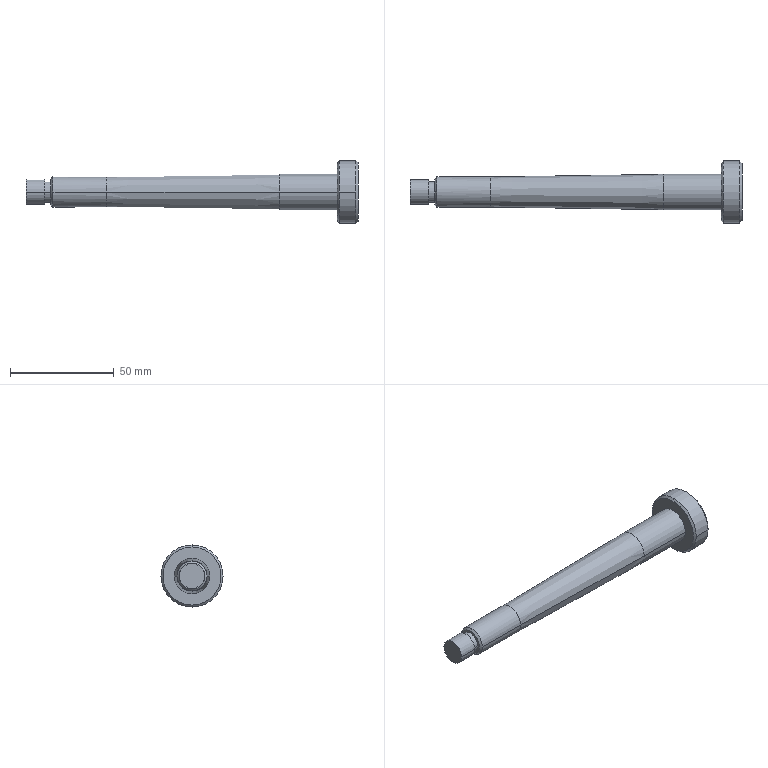Part | SolidWorks | features Chamfer 1, Revolution 1 | 1 solid | 23 faces | box 160 x 30 x 30 mm | volume 35227 mm3 | cylinder 10 | cone 8 | plane 5 | commonest cylinder face diameters 10 x2 12 x2 14.5 x2 17 x2 30 x2
STEP:
#1=CARTESIAN_POINT('',(272.45,-57.118,14.));
#2=VERTEX_POINT('',#1);
#3=CARTESIAN_POINT('',(272.45,-57.118,-14.));
#4=VERTEX_POINT('',#3);
#5=CARTESIAN_POINT('',(272.45,-57.118,0.));
#6=DIRECTION('',(-1.,0.,0.));
#7=DIRECTION('',(0.,-1.,0.));
#8=AXIS2_PLACEMENT_3D('',#5,#6,#7);
#9=CIRCLE('',#8,14.);
#10=EDGE_CURVE('',#2,#4,#9,.T.);
#11=ORIENTED_EDGE('',*,*,#10,.F.);
#12=CARTESIAN_POINT('',(273.45,-57.118,15.));
#13=VERTEX_POINT('',#12);
#14=CARTESIAN_POINT('',(273.45,-57.118,15.));
#15=DIRECTION('',(0.7071,0.,0.7071));
#16=VECTOR('',#15,1000.);
#17=LINE('',#14,#16);
#18=EDGE_CURVE('',#2,#13,#17,.T.);
#19=ORIENTED_EDGE('',*,*,#18,.T.);
#20=CARTESIAN_POINT('',(273.45,-42.118,0.));
#21=VERTEX_POINT('',#20);
#22=CARTESIAN_POINT('',(273.45,-57.118,0.));
#23=DIRECTION('',(1.,0.,0.));
#24=DIRECTION('',(0.,0.,1.));
#25=AXIS2_PLACEMENT_3D('',#22,#23,#24);
#26=CIRCLE('',#25,15.);
#27=EDGE_CURVE('',#21,#13,#26,.T.);
#28=ORIENTED_EDGE('',*,*,#27,.F.);
#29=CARTESIAN_POINT('',(273.45,-57.118,-15.));
#30=VERTEX_POINT('',#29);
#31=CARTESIAN_POINT('',(273.45,-57.118,0.));
#32=DIRECTION('',(1.,0.,0.));
#33=DIRECTION('',(0.,0.,1.));
#34=AXIS2_PLACEMENT_3D('',#31,#32,#33);
#35=CIRCLE('',#34,15.);
#36=EDGE_CURVE('',#30,#21,#35,.T.);
#37=ORIENTED_EDGE('',*,*,#36,.F.);
#38=CARTESIAN_POINT('',(273.45,-57.118,-15.));
#39=DIRECTION('',(0.7071,0.,-0.7071));
#40=VECTOR('',#39,1000.);
#41=LINE('',#38,#40);
#42=EDGE_CURVE('',#4,#30,#41,.T.);
#43=ORIENTED_EDGE('',*,*,#42,.F.);
#44=EDGE_LOOP('',(#11,#19,#28,#37,#43));
#45=FACE_OUTER_BOUND('',#44,.T.);
#46=CARTESIAN_POINT('',(273.45,-57.118,0.));
#47=DIRECTION('',(1.,0.,0.));
#48=DIRECTION('',(0.,0.,-1.));
#49=AXIS2_PLACEMENT_3D('',#46,#47,#48);
#50=CONICAL_SURFACE('',#49,15.,0.7854);
#51=ADVANCED_FACE('',(#45),#50,.T.);
#52=CARTESIAN_POINT('',(282.45,-57.118,-14.));
#53=VERTEX_POINT('',#52);
#54=CARTESIAN_POINT('',(282.45,-57.118,14.));
#55=VERTEX_POINT('',#54);
#56=CARTESIAN_POINT('',(282.45,-57.118,0.));
#57=DIRECTION('',(1.,0.,0.));
#58=DIRECTION('',(0.,1.,0.));
#59=AXIS2_PLACEMENT_3D('',#56,#57,#58);
#60=CIRCLE('',#59,14.);
#61=EDGE_CURVE('',#53,#55,#60,.T.);
#62=ORIENTED_EDGE('',*,*,#61,.F.);
#63=CARTESIAN_POINT('',(281.45,-57.118,-15.));
#64=VERTEX_POINT('',#63);
#65=CARTESIAN_POINT('',(282.45,-57.118,-14.));
#66=DIRECTION('',(-0.7071,0.,-0.7071));
#67=VECTOR('',#66,1000.);
#68=LINE('',#65,#67);
#69=EDGE_CURVE('',#53,#64,#68,.T.);
#70=ORIENTED_EDGE('',*,*,#69,.T.);
#71=CARTESIAN_POINT('',(281.45,-42.118,0.));
#72=VERTEX_POINT('',#71);
#73=CARTESIAN_POINT('',(281.45,-57.118,0.));
#74=DIRECTION('',(-1.,0.,0.));
#75=DIRECTION('',(0.,0.,-1.));
#76=AXIS2_PLACEMENT_3D('',#73,#74,#75);
#77=CIRCLE('',#76,15.);
#78=EDGE_CURVE('',#72,#64,#77,.T.);
#79=ORIENTED_EDGE('',*,*,#78,.F.);
#80=CARTESIAN_POINT('',(281.45,-57.118,15.));
#81=VERTEX_POINT('',#80);
#82=CARTESIAN_POINT('',(281.45,-57.118,0.));
#83=DIRECTION('',(-1.,0.,0.));
#84=DIRECTION('',(0.,0.,-1.));
#85=AXIS2_PLACEMENT_3D('',#82,#83,#84);
#86=CIRCLE('',#85,15.);
#87=EDGE_CURVE('',#81,#72,#86,.T.);
#88=ORIENTED_EDGE('',*,*,#87,.F.);
#89=CARTESIAN_POINT('',(282.45,-57.118,14.));
#90=DIRECTION('',(-0.7071,0.,0.7071));
#91=VECTOR('',#90,1000.);
#92=LINE('',#89,#91);
#93=EDGE_CURVE('',#55,#81,#92,.T.);
#94=ORIENTED_EDGE('',*,*,#93,.F.);
#95=EDGE_LOOP('',(#62,#70,#79,#88,#94));
#96=FACE_OUTER_BOUND('',#95,.T.);
#97=CARTESIAN_POINT('',(282.45,-57.118,0.));
#98=DIRECTION('',(-1.,0.,0.));
#99=DIRECTION('',(0.,0.,1.));
#100=AXIS2_PLACEMENT_3D('',#97,#98,#99);
#101=CONICAL_SURFACE('',#100,14.,0.7854);
#102=ADVANCED_FACE('',(#96),#101,.T.);
#103=CARTESIAN_POINT('',(134.45,-57.118,6.25));
#104=VERTEX_POINT('',#103);
#105=CARTESIAN_POINT('',(134.45,-57.118,-6.25));
#106=VERTEX_POINT('',#105);
#107=CARTESIAN_POINT('',(134.45,-57.118,0.));
#108=DIRECTION('',(-1.,0.,0.));
#109=DIRECTION('',(0.,-1.,0.));
#110=AXIS2_PLACEMENT_3D('',#107,#108,#109);
#111=CIRCLE('',#110,6.25);
#112=EDGE_CURVE('',#104,#106,#111,.T.);
#113=ORIENTED_EDGE('',*,*,#112,.F.);
#114=CARTESIAN_POINT('',(135.45,-57.118,7.25));
#115=VERTEX_POINT('',#114);
#116=CARTESIAN_POINT('',(135.45,-57.118,7.25));
#117=DIRECTION('',(0.7071,0.,0.7071));
#118=VECTOR('',#117,1000.);
#119=LINE('',#116,#118);
#120=EDGE_CURVE('',#104,#115,#119,.T.);
#121=ORIENTED_EDGE('',*,*,#120,.T.);
#122=CARTESIAN_POINT('',(135.45,-49.868,0.));
#123=VERTEX_POINT('',#122);
#124=CARTESIAN_POINT('',(135.45,-57.118,0.));
#125=DIRECTION('',(1.,0.,0.));
#126=DIRECTION('',(0.,0.,1.));
#127=AXIS2_PLACEMENT_3D('',#124,#125,#126);
#128=CIRCLE('',#127,7.25);
#129=EDGE_CURVE('',#123,#115,#128,.T.);
#130=ORIENTED_EDGE('',*,*,#129,.F.);
#131=CARTESIAN_POINT('',(135.45,-57.118,-7.25));
#132=VERTEX_POINT('',#131);
#133=CARTESIAN_POINT('',(135.45,-57.118,0.));
#134=DIRECTION('',(1.,0.,0.));
#135=DIRECTION('',(0.,0.,1.));
#136=AXIS2_PLACEMENT_3D('',#133,#134,#135);
#137=CIRCLE('',#136,7.25);
#138=EDGE_CURVE('',#132,#123,#137,.T.);
#139=ORIENTED_EDGE('',*,*,#138,.F.);
#140=CARTESIAN_POINT('',(135.45,-57.118,-7.25));
#141=DIRECTION('',(0.7071,0.,-0.7071));
#142=VECTOR('',#141,1000.);
#143=LINE('',#140,#142);
#144=EDGE_CURVE('',#106,#132,#143,.T.);
#145=ORIENTED_EDGE('',*,*,#144,.F.);
#146=EDGE_LOOP('',(#113,#121,#130,#139,#145));
#147=FACE_OUTER_BOUND('',#146,.T.);
#148=CARTESIAN_POINT('',(135.45,-57.118,0.));
#149=DIRECTION('',(1.,0.,0.));
#150=DIRECTION('',(0.,0.,-1.));
#151=AXIS2_PLACEMENT_3D('',#148,#149,#150);
#152=CONICAL_SURFACE('',#151,7.25,0.7854);
#153=ADVANCED_FACE('',(#147),#152,.T.);
#154=CARTESIAN_POINT('',(131.45,-52.118,0.));
#155=VERTEX_POINT('',#154);
#156=CARTESIAN_POINT('',(131.45,-62.118,0.));
#157=VERTEX_POINT('',#156);
#158=CARTESIAN_POINT('',(131.45,-57.118,0.));
#159=DIRECTION('',(1.,0.,0.));
#160=DIRECTION('',(0.,1.,0.));
#161=AXIS2_PLACEMENT_3D('',#158,#159,#160);
#162=CIRCLE('',#161,5.);
#163=EDGE_CURVE('',#155,#157,#162,.T.);
#164=ORIENTED_EDGE('',*,*,#163,.T.);
#165=CARTESIAN_POINT('',(134.45,-62.118,0.));
#166=VERTEX_POINT('',#165);
#167=CARTESIAN_POINT('',(272.45,-62.118,0.));
#168=DIRECTION('',(1.,0.,0.));
#169=VECTOR('',#168,1000.);
#170=LINE('',#167,#169);
#171=EDGE_CURVE('',#157,#166,#170,.T.);
#172=ORIENTED_EDGE('',*,*,#171,.T.);
#173=CARTESIAN_POINT('',(134.45,-52.118,0.));
#174=VERTEX_POINT('',#173);
#175=CARTESIAN_POINT('',(134.45,-57.118,0.));
#176=DIRECTION('',(1.,0.,0.));
#177=DIRECTION('',(0.,1.,0.));
#178=AXIS2_PLACEMENT_3D('',#175,#176,#177);
#179=CIRCLE('',#178,5.);
#180=EDGE_CURVE('',#174,#166,#179,.T.);
#181=ORIENTED_EDGE('',*,*,#180,.F.);
#182=CARTESIAN_POINT('',(272.45,-52.118,0.));
#183=DIRECTION('',(1.,0.,0.));
#184=VECTOR('',#183,1000.);
#185=LINE('',#182,#184);
#186=EDGE_CURVE('',#155,#174,#185,.T.);
#187=ORIENTED_EDGE('',*,*,#186,.F.);
#188=EDGE_LOOP('',(#164,#172,#181,#187));
#189=FACE_OUTER_BOUND('',#188,.T.);
#190=CARTESIAN_POINT('',(272.45,-57.118,0.));
#191=DIRECTION('',(1.,0.,0.));
#192=DIRECTION('',(0.,1.,0.));
#193=AXIS2_PLACEMENT_3D('',#190,#191,#192);
#194=CYLINDRICAL_SURFACE('',#193,5.);
#195=ADVANCED_FACE('',(#189),#194,.T.);
#196=CARTESIAN_POINT('',(122.45,-51.118,0.));
#197=VERTEX_POINT('',#196);
#198=CARTESIAN_POINT('',(122.45,-63.118,0.));
#199=VERTEX_POINT('',#198);
#200=CARTESIAN_POINT('',(122.45,-57.118,0.));
#201=DIRECTION('',(1.,0.,0.));
#202=DIRECTION('',(0.,1.,0.));
#203=AXIS2_PLACEMENT_3D('',#200,#201,#202);
#204=CIRCLE('',#203,6.);
#205=EDGE_CURVE('',#197,#199,#204,.T.);
#206=ORIENTED_EDGE('',*,*,#205,.T.);
#207=CARTESIAN_POINT('',(131.45,-63.118,0.));
#208=VERTEX_POINT('',#207);
#209=CARTESIAN_POINT('',(272.45,-63.118,0.));
#210=DIRECTION('',(1.,0.,0.));
#211=VECTOR('',#210,1000.);
#212=LINE('',#209,#211);
#213=EDGE_CURVE('',#199,#208,#212,.T.);
#214=ORIENTED_EDGE('',*,*,#213,.T.);
#215=CARTESIAN_POINT('',(131.45,-51.118,0.));
#216=VERTEX_POINT('',#215);
#217=CARTESIAN_POINT('',(131.45,-57.118,0.));
#218=DIRECTION('',(1.,0.,0.));
#219=DIRECTION('',(0.,1.,0.));
#220=AXIS2_PLACEMENT_3D('',#217,#218,#219);
#221=CIRCLE('',#220,6.);
#222=EDGE_CURVE('',#216,#208,#221,.T.);
#223=ORIENTED_EDGE('',*,*,#222,.F.);
#224=CARTESIAN_POINT('',(272.45,-51.118,0.));
#225=DIRECTION('',(1.,0.,0.));
#226=VECTOR('',#225,1000.);
#227=LINE('',#224,#226);
#228=EDGE_CURVE('',#197,#216,#227,.T.);
#229=ORIENTED_EDGE('',*,*,#228,.F.);
#230=EDGE_LOOP('',(#206,#214,#223,#229));
#231=FACE_OUTER_BOUND('',#230,.T.);
#232=CARTESIAN_POINT('',(272.45,-57.118,0.));
#233=DIRECTION('',(1.,0.,0.));
#234=DIRECTION('',(0.,1.,0.));
#235=AXIS2_PLACEMENT_3D('',#232,#233,#234);
#236=CYLINDRICAL_SURFACE('',#235,6.);
#237=ADVANCED_FACE('',(#231),#236,.T.);
#238=ORIENTED_EDGE('',*,*,#27,.T.);
#239=CARTESIAN_POINT('',(273.45,-72.118,0.));
#240=VERTEX_POINT('',#239);
#241=CARTESIAN_POINT('',(273.45,-57.118,0.));
#242=DIRECTION('',(1.,0.,0.));
#243=DIRECTION('',(0.,0.,1.));
#244=AXIS2_PLACEMENT_3D('',#241,#242,#243);
#245=CIRCLE('',#244,15.);
#246=EDGE_CURVE('',#13,#240,#245,.T.);
#247=ORIENTED_EDGE('',*,*,#246,.T.);
#248=CARTESIAN_POINT('',(281.45,-72.118,0.));
#249=VERTEX_POINT('',#248);
#250=CARTESIAN_POINT('',(272.45,-72.118,0.));
#251=DIRECTION('',(1.,0.,0.));
#252=VECTOR('',#251,1000.);
#253=LINE('',#250,#252);
#254=EDGE_CURVE('',#240,#249,#253,.T.);
#255=ORIENTED_EDGE('',*,*,#254,.T.);
#256=CARTESIAN_POINT('',(281.45,-57.118,0.));
#257=DIRECTION('',(-1.,0.,0.));
#258=DIRECTION('',(0.,0.,-1.));
#259=AXIS2_PLACEMENT_3D('',#256,#257,#258);
#260=CIRCLE('',#259,15.);
#261=EDGE_CURVE('',#249,#81,#260,.T.);
#262=ORIENTED_EDGE('',*,*,#261,.T.);
#263=ORIENTED_EDGE('',*,*,#87,.T.);
#264=CARTESIAN_POINT('',(272.45,-42.118,0.));
#265=DIRECTION('',(1.,0.,0.));
#266=VECTOR('',#265,1000.);
#267=LINE('',#264,#266);
#268=EDGE_CURVE('',#21,#72,#267,.T.);
#269=ORIENTED_EDGE('',*,*,#268,.F.);
#270=EDGE_LOOP('',(#238,#247,#255,#262,#263,#269));
#271=FACE_OUTER_BOUND('',#270,.T.);
#272=CARTESIAN_POINT('',(272.45,-57.118,0.));
#273=DIRECTION('',(1.,0.,0.));
#274=DIRECTION('',(0.,1.,0.));
#275=AXIS2_PLACEMENT_3D('',#272,#273,#274);
#276=CYLINDRICAL_SURFACE('',#275,15.);
#277=ADVANCED_FACE('',(#271),#276,.T.);
#278=CARTESIAN_POINT('',(244.45,-48.618,0.));
#279=VERTEX_POINT('',#278);
#280=CARTESIAN_POINT('',(244.45,-65.618,0.));
#281=VERTEX_POINT('',#280);
#282=CARTESIAN_POINT('',(244.45,-57.118,0.));
#283=DIRECTION('',(1.,0.,0.));
#284=DIRECTION('',(0.,1.,0.));
#285=AXIS2_PLACEMENT_3D('',#282,#283,#284);
#286=CIRCLE('',#285,8.5);
#287=EDGE_CURVE('',#279,#281,#286,.T.);
#288=ORIENTED_EDGE('',*,*,#287,.T.);
#289=CARTESIAN_POINT('',(272.45,-65.618,0.));
#290=VERTEX_POINT('',#289);
#291=CARTESIAN_POINT('',(272.45,-65.618,0.));
#292=DIRECTION('',(1.,0.,0.));
#293=VECTOR('',#292,1000.);
#294=LINE('',#291,#293);
#295=EDGE_CURVE('',#281,#290,#294,.T.);
#296=ORIENTED_EDGE('',*,*,#295,.T.);
#297=CARTESIAN_POINT('',(272.45,-48.618,0.));
#298=VERTEX_POINT('',#297);
#299=CARTESIAN_POINT('',(272.45,-57.118,0.));
#300=DIRECTION('',(1.,0.,0.));
#301=DIRECTION('',(0.,1.,0.));
#302=AXIS2_PLACEMENT_3D('',#299,#300,#301);
#303=CIRCLE('',#302,8.5);
#304=EDGE_CURVE('',#298,#290,#303,.T.);
#305=ORIENTED_EDGE('',*,*,#304,.F.);
#306=CARTESIAN_POINT('',(272.45,-48.618,0.));
#307=DIRECTION('',(1.,0.,0.));
#308=VECTOR('',#307,1000.);
#309=LINE('',#306,#308);
#310=EDGE_CURVE('',#279,#298,#309,.T.);
#311=ORIENTED_EDGE('',*,*,#310,.F.);
#312=EDGE_LOOP('',(#288,#296,#305,#311));
#313=FACE_OUTER_BOUND('',#312,.T.);
#314=CARTESIAN_POINT('',(272.45,-57.118,0.));
#315=DIRECTION('',(1.,0.,0.));
#316=DIRECTION('',(0.,1.,0.));
#317=AXIS2_PLACEMENT_3D('',#314,#315,#316);
#318=CYLINDRICAL_SURFACE('',#317,8.5);
#319=ADVANCED_FACE('',(#313),#318,.T.);
#320=CARTESIAN_POINT('',(161.45,-49.868,0.));
#321=VERTEX_POINT('',#320);
#322=CARTESIAN_POINT('',(161.45,-64.368,0.));
#323=VERTEX_POINT('',#322);
#324=CARTESIAN_POINT('',(161.45,-57.118,0.));
#325=DIRECTION('',(1.,0.,0.));
#326=DIRECTION('',(0.,1.,0.));
#327=AXIS2_PLACEMENT_3D('',#324,#325,#326);
#328=CIRCLE('',#327,7.25);
#329=EDGE_CURVE('',#321,#323,#328,.T.);
#330=ORIENTED_EDGE('',*,*,#329,.T.);
#331=CARTESIAN_POINT('',(244.45,-65.618,0.));
#332=DIRECTION('',(0.9999,-0.01506,0.));
#333=VECTOR('',#332,1000.);
#334=LINE('',#331,#333);
#335=EDGE_CURVE('',#323,#281,#334,.T.);
#336=ORIENTED_EDGE('',*,*,#335,.T.);
#337=ORIENTED_EDGE('',*,*,#287,.F.);
#338=CARTESIAN_POINT('',(244.45,-48.618,0.));
#339=DIRECTION('',(0.9999,0.01506,0.));
#340=VECTOR('',#339,1000.);
#341=LINE('',#338,#340);
#342=EDGE_CURVE('',#321,#279,#341,.T.);
#343=ORIENTED_EDGE('',*,*,#342,.F.);
#344=EDGE_LOOP('',(#330,#336,#337,#343));
#345=FACE_OUTER_BOUND('',#344,.T.);
#346=CARTESIAN_POINT('',(244.45,-57.118,0.));
#347=DIRECTION('',(1.,0.,0.));
#348=DIRECTION('',(0.,1.,0.));
#349=AXIS2_PLACEMENT_3D('',#346,#347,#348);
#350=CONICAL_SURFACE('',#349,8.5,0.01506);
#351=ADVANCED_FACE('',(#345),#350,.T.);
#352=ORIENTED_EDGE('',*,*,#129,.T.);
#353=CARTESIAN_POINT('',(135.45,-64.368,0.));
#354=VERTEX_POINT('',#353);
#355=CARTESIAN_POINT('',(135.45,-57.118,0.));
#356=DIRECTION('',(1.,0.,0.));
#357=DIRECTION('',(0.,0.,1.));
#358=AXIS2_PLACEMENT_3D('',#355,#356,#357);
#359=CIRCLE('',#358,7.25);
#360=EDGE_CURVE('',#115,#354,#359,.T.);
#361=ORIENTED_EDGE('',*,*,#360,.T.);
#362=CARTESIAN_POINT('',(272.45,-64.368,0.));
#363=DIRECTION('',(1.,0.,0.));
#364=VECTOR('',#363,1000.);
#365=LINE('',#362,#364);
#366=EDGE_CURVE('',#354,#323,#365,.T.);
#367=ORIENTED_EDGE('',*,*,#366,.T.);
#368=ORIENTED_EDGE('',*,*,#329,.F.);
#369=CARTESIAN_POINT('',(272.45,-49.868,0.));
#370=DIRECTION('',(1.,0.,0.));
#371=VECTOR('',#370,1000.);
#372=LINE('',#369,#371);
#373=EDGE_CURVE('',#123,#321,#372,.T.);
#374=ORIENTED_EDGE('',*,*,#373,.F.);
#375=EDGE_LOOP('',(#352,#361,#367,#368,#374));
#376=FACE_OUTER_BOUND('',#375,.T.);
#377=CARTESIAN_POINT('',(272.45,-57.118,0.));
#378=DIRECTION('',(1.,0.,0.));
#379=DIRECTION('',(0.,1.,0.));
#380=AXIS2_PLACEMENT_3D('',#377,#378,#379);
#381=CYLINDRICAL_SURFACE('',#380,7.25);
#382=ADVANCED_FACE('',(#376),#381,.T.);
#383=CARTESIAN_POINT('',(134.45,-57.118,0.));
#384=DIRECTION('',(-1.,0.,0.));
#385=DIRECTION('',(0.,-1.,0.));
#386=AXIS2_PLACEMENT_3D('',#383,#384,#385);
#387=CIRCLE('',#386,6.25);
#388=EDGE_CURVE('',#106,#104,#387,.T.);
#389=ORIENTED_EDGE('',*,*,#388,.T.);
#390=ORIENTED_EDGE('',*,*,#112,.T.);
#391=EDGE_LOOP('',(#389,#390));
#392=FACE_OUTER_BOUND('',#391,.T.);
#393=ORIENTED_EDGE('',*,*,#180,.T.);
#394=CARTESIAN_POINT('',(134.45,-57.118,0.));
#395=DIRECTION('',(1.,0.,0.));
#396=DIRECTION('',(0.,1.,0.));
#397=AXIS2_PLACEMENT_3D('',#394,#395,#396);
#398=CIRCLE('',#397,5.);
#399=EDGE_CURVE('',#166,#174,#398,.T.);
#400=ORIENTED_EDGE('',*,*,#399,.T.);
#401=EDGE_LOOP('',(#393,#400));
#402=FACE_BOUND('',#401,.T.);
#403=CARTESIAN_POINT('',(134.45,-49.868,0.));
#404=DIRECTION('',(-1.,0.,0.));
#405=DIRECTION('',(0.,-1.,0.));
#406=AXIS2_PLACEMENT_3D('',#403,#404,#405);
#407=PLANE('',#406);
#408=ADVANCED_FACE('',(#392,#402),#407,.T.);
#409=ORIENTED_EDGE('',*,*,#366,.F.);
#410=CARTESIAN_POINT('',(135.45,-57.118,0.));
#411=DIRECTION('',(1.,0.,0.));
#412=DIRECTION('',(0.,0.,1.));
#413=AXIS2_PLACEMENT_3D('',#410,#411,#412);
#414=CIRCLE('',#413,7.25);
#415=EDGE_CURVE('',#354,#132,#414,.T.);
#416=ORIENTED_EDGE('',*,*,#415,.T.);
#417=ORIENTED_EDGE('',*,*,#138,.T.);
#418=ORIENTED_EDGE('',*,*,#373,.T.);
#419=CARTESIAN_POINT('',(161.45,-57.118,0.));
#420=DIRECTION('',(1.,0.,0.));
#421=DIRECTION('',(0.,1.,0.));
#422=AXIS2_PLACEMENT_3D('',#419,#420,#421);
#423=CIRCLE('',#422,7.25);
#424=EDGE_CURVE('',#323,#321,#423,.T.);
#425=ORIENTED_EDGE('',*,*,#424,.F.);
#426=EDGE_LOOP('',(#409,#416,#417,#418,#425));
#427=FACE_OUTER_BOUND('',#426,.T.);
#428=CARTESIAN_POINT('',(272.45,-57.118,0.));
#429=DIRECTION('',(1.,0.,0.));
#430=DIRECTION('',(0.,1.,0.));
#431=AXIS2_PLACEMENT_3D('',#428,#429,#430);
#432=CYLINDRICAL_SURFACE('',#431,7.25);
#433=ADVANCED_FACE('',(#427),#432,.T.);
#434=ORIENTED_EDGE('',*,*,#335,.F.);
#435=ORIENTED_EDGE('',*,*,#424,.T.);
#436=ORIENTED_EDGE('',*,*,#342,.T.);
#437=CARTESIAN_POINT('',(244.45,-57.118,0.));
#438=DIRECTION('',(1.,0.,0.));
#439=DIRECTION('',(0.,1.,0.));
#440=AXIS2_PLACEMENT_3D('',#437,#438,#439);
#441=CIRCLE('',#440,8.5);
#442=EDGE_CURVE('',#281,#279,#441,.T.);
#443=ORIENTED_EDGE('',*,*,#442,.F.);
#444=EDGE_LOOP('',(#434,#435,#436,#443));
#445=FACE_OUTER_BOUND('',#444,.T.);
#446=CARTESIAN_POINT('',(244.45,-57.118,0.));
#447=DIRECTION('',(1.,0.,0.));
#448=DIRECTION('',(0.,1.,0.));
#449=AXIS2_PLACEMENT_3D('',#446,#447,#448);
#450=CONICAL_SURFACE('',#449,8.5,0.01506);
#451=ADVANCED_FACE('',(#445),#450,.T.);
#452=ORIENTED_EDGE('',*,*,#295,.F.);
#453=ORIENTED_EDGE('',*,*,#442,.T.);
#454=ORIENTED_EDGE('',*,*,#310,.T.);
#455=CARTESIAN_POINT('',(272.45,-57.118,0.));
#456=DIRECTION('',(1.,0.,0.));
#457=DIRECTION('',(0.,1.,0.));
#458=AXIS2_PLACEMENT_3D('',#455,#456,#457);
#459=CIRCLE('',#458,8.5);
#460=EDGE_CURVE('',#290,#298,#459,.T.);
#461=ORIENTED_EDGE('',*,*,#460,.F.);
#462=EDGE_LOOP('',(#452,#453,#454,#461));
#463=FACE_OUTER_BOUND('',#462,.T.);
#464=CARTESIAN_POINT('',(272.45,-57.118,0.));
#465=DIRECTION('',(1.,0.,0.));
#466=DIRECTION('',(0.,1.,0.));
#467=AXIS2_PLACEMENT_3D('',#464,#465,#466);
#468=CYLINDRICAL_SURFACE('',#467,8.5);
#469=ADVANCED_FACE('',(#463),#468,.T.);
#470=CARTESIAN_POINT('',(272.45,-57.118,0.));
#471=DIRECTION('',(-1.,0.,0.));
#472=DIRECTION('',(0.,-1.,0.));
#473=AXIS2_PLACEMENT_3D('',#470,#471,#472);
#474=CIRCLE('',#473,14.);
#475=EDGE_CURVE('',#4,#2,#474,.T.);
#476=ORIENTED_EDGE('',*,*,#475,.T.);
#477=ORIENTED_EDGE('',*,*,#10,.T.);
#478=EDGE_LOOP('',(#476,#477));
#479=FACE_OUTER_BOUND('',#478,.T.);
#480=ORIENTED_EDGE('',*,*,#304,.T.);
#481=ORIENTED_EDGE('',*,*,#460,.T.);
#482=EDGE_LOOP('',(#480,#481));
#483=FACE_BOUND('',#482,.T.);
#484=CARTESIAN_POINT('',(272.45,-48.618,0.));
#485=DIRECTION('',(-1.,0.,0.));
#486=DIRECTION('',(0.,-1.,0.));
#487=AXIS2_PLACEMENT_3D('',#484,#485,#486);
#488=PLANE('',#487);
#489=ADVANCED_FACE('',(#479,#483),#488,.T.);
#490=ORIENTED_EDGE('',*,*,#254,.F.);
#491=CARTESIAN_POINT('',(273.45,-57.118,0.));
#492=DIRECTION('',(1.,0.,0.));
#493=DIRECTION('',(0.,0.,1.));
#494=AXIS2_PLACEMENT_3D('',#491,#492,#493);
#495=CIRCLE('',#494,15.);
#496=EDGE_CURVE('',#240,#30,#495,.T.);
#497=ORIENTED_EDGE('',*,*,#496,.T.);
#498=ORIENTED_EDGE('',*,*,#36,.T.);
#499=ORIENTED_EDGE('',*,*,#268,.T.);
#500=ORIENTED_EDGE('',*,*,#78,.T.);
#501=CARTESIAN_POINT('',(281.45,-57.118,0.));
#502=DIRECTION('',(-1.,0.,0.));
#503=DIRECTION('',(0.,0.,-1.));
#504=AXIS2_PLACEMENT_3D('',#501,#502,#503);
#505=CIRCLE('',#504,15.);
#506=EDGE_CURVE('',#64,#249,#505,.T.);
#507=ORIENTED_EDGE('',*,*,#506,.T.);
#508=EDGE_LOOP('',(#490,#497,#498,#499,#500,#507));
#509=FACE_OUTER_BOUND('',#508,.T.);
#510=CARTESIAN_POINT('',(272.45,-57.118,0.));
#511=DIRECTION('',(1.,0.,0.));
#512=DIRECTION('',(0.,1.,0.));
#513=AXIS2_PLACEMENT_3D('',#510,#511,#512);
#514=CYLINDRICAL_SURFACE('',#513,15.);
#515=ADVANCED_FACE('',(#509),#514,.T.);
#516=CARTESIAN_POINT('',(282.45,-57.118,0.));
#517=DIRECTION('',(1.,0.,0.));
#518=DIRECTION('',(0.,1.,0.));
#519=AXIS2_PLACEMENT_3D('',#516,#517,#518);
#520=CIRCLE('',#519,14.);
#521=EDGE_CURVE('',#55,#53,#520,.T.);
#522=ORIENTED_EDGE('',*,*,#521,.T.);
#523=ORIENTED_EDGE('',*,*,#61,.T.);
#524=EDGE_LOOP('',(#522,#523));
#525=FACE_OUTER_BOUND('',#524,.T.);
#526=CARTESIAN_POINT('',(282.45,-42.118,0.));
#527=DIRECTION('',(1.,0.,0.));
#528=DIRECTION('',(0.,1.,0.));
#529=AXIS2_PLACEMENT_3D('',#526,#527,#528);
#530=PLANE('',#529);
#531=ADVANCED_FACE('',(#525),#530,.T.);
#532=ORIENTED_EDGE('',*,*,#205,.F.);
#533=CARTESIAN_POINT('',(122.45,-57.118,0.));
#534=DIRECTION('',(1.,0.,0.));
#535=DIRECTION('',(0.,1.,0.));
#536=AXIS2_PLACEMENT_3D('',#533,#534,#535);
#537=CIRCLE('',#536,6.);
#538=EDGE_CURVE('',#199,#197,#537,.T.);
#539=ORIENTED_EDGE('',*,*,#538,.F.);
#540=EDGE_LOOP('',(#532,#539));
#541=FACE_OUTER_BOUND('',#540,.T.);
#542=CARTESIAN_POINT('',(122.45,-51.118,0.));
#543=DIRECTION('',(-1.,0.,0.));
#544=DIRECTION('',(0.,-1.,0.));
#545=AXIS2_PLACEMENT_3D('',#542,#543,#544);
#546=PLANE('',#545);
#547=ADVANCED_FACE('',(#541),#546,.T.);
#548=ORIENTED_EDGE('',*,*,#213,.F.);
#549=ORIENTED_EDGE('',*,*,#538,.T.);
#550=ORIENTED_EDGE('',*,*,#228,.T.);
#551=CARTESIAN_POINT('',(131.45,-57.118,0.));
#552=DIRECTION('',(1.,0.,0.));
#553=DIRECTION('',(0.,1.,0.));
#554=AXIS2_PLACEMENT_3D('',#551,#552,#553);
#555=CIRCLE('',#554,6.);
#556=EDGE_CURVE('',#208,#216,#555,.T.);
#557=ORIENTED_EDGE('',*,*,#556,.F.);
#558=EDGE_LOOP('',(#548,#549,#550,#557));
#559=FACE_OUTER_BOUND('',#558,.T.);
#560=CARTESIAN_POINT('',(272.45,-57.118,0.));
#561=DIRECTION('',(1.,0.,0.));
#562=DIRECTION('',(0.,1.,0.));
#563=AXIS2_PLACEMENT_3D('',#560,#561,#562);
#564=CYLINDRICAL_SURFACE('',#563,6.);
#565=ADVANCED_FACE('',(#559),#564,.T.);
#566=ORIENTED_EDGE('',*,*,#222,.T.);
#567=ORIENTED_EDGE('',*,*,#556,.T.);
#568=EDGE_LOOP('',(#566,#567));
#569=FACE_OUTER_BOUND('',#568,.T.);
#570=ORIENTED_EDGE('',*,*,#163,.F.);
#571=CARTESIAN_POINT('',(131.45,-57.118,0.));
#572=DIRECTION('',(1.,0.,0.));
#573=DIRECTION('',(0.,1.,0.));
#574=AXIS2_PLACEMENT_3D('',#571,#572,#573);
#575=CIRCLE('',#574,5.);
#576=EDGE_CURVE('',#157,#155,#575,.T.);
#577=ORIENTED_EDGE('',*,*,#576,.F.);
#578=EDGE_LOOP('',(#570,#577));
#579=FACE_BOUND('',#578,.T.);
#580=CARTESIAN_POINT('',(131.45,-52.118,0.));
#581=DIRECTION('',(1.,0.,0.));
#582=DIRECTION('',(0.,1.,0.));
#583=AXIS2_PLACEMENT_3D('',#580,#581,#582);
#584=PLANE('',#583);
#585=ADVANCED_FACE('',(#569,#579),#584,.T.);
#586=ORIENTED_EDGE('',*,*,#171,.F.);
#587=ORIENTED_EDGE('',*,*,#576,.T.);
#588=ORIENTED_EDGE('',*,*,#186,.T.);
#589=ORIENTED_EDGE('',*,*,#399,.F.);
#590=EDGE_LOOP('',(#586,#587,#588,#589));
#591=FACE_OUTER_BOUND('',#590,.T.);
#592=CARTESIAN_POINT('',(272.45,-57.118,0.));
#593=DIRECTION('',(1.,0.,0.));
#594=DIRECTION('',(0.,1.,0.));
#595=AXIS2_PLACEMENT_3D('',#592,#593,#594);
#596=CYLINDRICAL_SURFACE('',#595,5.);
#597=ADVANCED_FACE('',(#591),#596,.T.);
#598=ORIENTED_EDGE('',*,*,#120,.F.);
#599=ORIENTED_EDGE('',*,*,#388,.F.);
#600=ORIENTED_EDGE('',*,*,#144,.T.);
#601=ORIENTED_EDGE('',*,*,#415,.F.);
#602=ORIENTED_EDGE('',*,*,#360,.F.);
#603=EDGE_LOOP('',(#598,#599,#600,#601,#602));
#604=FACE_OUTER_BOUND('',#603,.T.);
#605=CARTESIAN_POINT('',(135.45,-57.118,0.));
#606=DIRECTION('',(1.,0.,0.));
#607=DIRECTION('',(0.,0.,-1.));
#608=AXIS2_PLACEMENT_3D('',#605,#606,#607);
#609=CONICAL_SURFACE('',#608,7.25,0.7854);
#610=ADVANCED_FACE('',(#604),#609,.T.);
#611=ORIENTED_EDGE('',*,*,#69,.F.);
#612=ORIENTED_EDGE('',*,*,#521,.F.);
#613=ORIENTED_EDGE('',*,*,#93,.T.);
#614=ORIENTED_EDGE('',*,*,#261,.F.);
#615=ORIENTED_EDGE('',*,*,#506,.F.);
#616=EDGE_LOOP('',(#611,#612,#613,#614,#615));
#617=FACE_OUTER_BOUND('',#616,.T.);
#618=CARTESIAN_POINT('',(282.45,-57.118,0.));
#619=DIRECTION('',(-1.,0.,0.));
#620=DIRECTION('',(0.,0.,1.));
#621=AXIS2_PLACEMENT_3D('',#618,#619,#620);
#622=CONICAL_SURFACE('',#621,14.,0.7854);
#623=ADVANCED_FACE('',(#617),#622,.T.);
#624=ORIENTED_EDGE('',*,*,#18,.F.);
#625=ORIENTED_EDGE('',*,*,#475,.F.);
#626=ORIENTED_EDGE('',*,*,#42,.T.);
#627=ORIENTED_EDGE('',*,*,#496,.F.);
#628=ORIENTED_EDGE('',*,*,#246,.F.);
#629=EDGE_LOOP('',(#624,#625,#626,#627,#628));
#630=FACE_OUTER_BOUND('',#629,.T.);
#631=CARTESIAN_POINT('',(273.45,-57.118,0.));
#632=DIRECTION('',(1.,0.,0.));
#633=DIRECTION('',(0.,0.,-1.));
#634=AXIS2_PLACEMENT_3D('',#631,#632,#633);
#635=CONICAL_SURFACE('',#634,15.,0.7854);
#636=ADVANCED_FACE('',(#630),#635,.T.);
#637=CLOSED_SHELL('',(#51,#102,#153,#195,#237,#277,#319,#351,#382,#408,#433,#451,#469,#489,#515,#531,#547,#565,#585,#597,#610,#623,#636));
#638=MANIFOLD_SOLID_BREP('',#637);
#639=CARTESIAN_POINT('',(0.,0.,0.));
#640=DIRECTION('',(0.,0.,1.));
#641=DIRECTION('',(1.,0.,0.));
#642=AXIS2_PLACEMENT_3D('',#639,#640,#641);
#643=(LENGTH_UNIT()NAMED_UNIT(*)SI_UNIT(.MILLI.,.METRE.));
#644=UNCERTAINTY_MEASURE_WITH_UNIT(LENGTH_MEASURE(0.00001),#643,'','');
#645=(NAMED_UNIT(*)PLANE_ANGLE_UNIT()SI_UNIT($,.RADIAN.));
#646=(NAMED_UNIT(*)SI_UNIT($,.STERADIAN.)SOLID_ANGLE_UNIT());
#647=(GEOMETRIC_REPRESENTATION_CONTEXT(3)GLOBAL_UNCERTAINTY_ASSIGNED_CONTEXT((#644))GLOBAL_UNIT_ASSIGNED_CONTEXT((#643,#645,#646))REPRESENTATION_CONTEXT('',''));
#648=ADVANCED_BREP_SHAPE_REPRESENTATION('',(#638,#642),#647);